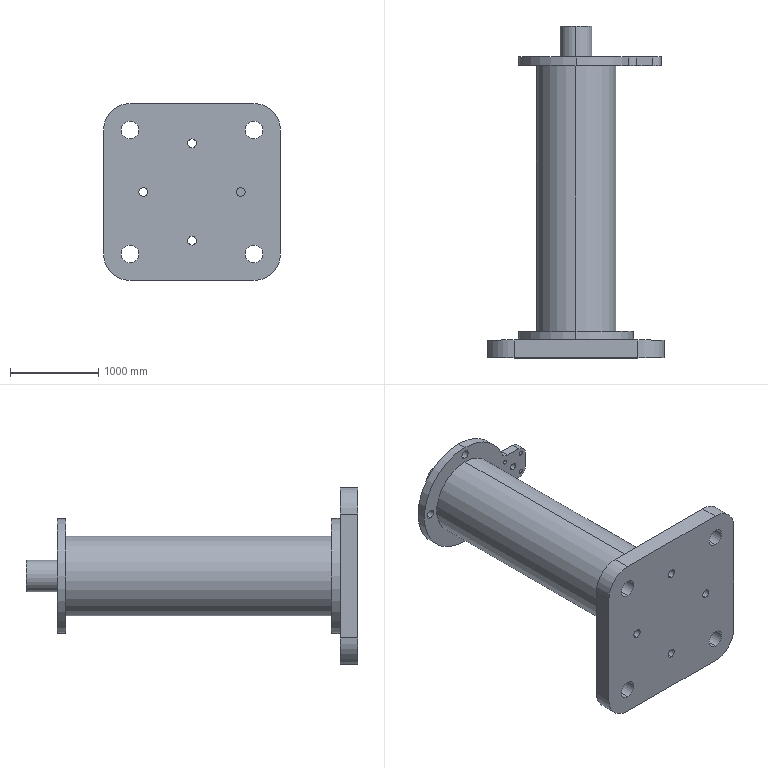Part | SolidWorks | features ICE 8, Extrusion 1, Fillet 1, MirrorPattern 1 | 1 solid | 62 faces | box 2000 x 3750 x 2000 mm | volume 2968644378 mm3 | cylinder 49 | plane 13 | commonest cylinder face diameters 100 x14 200 x12 50 x8 1300 x5 600 x4 80 x2